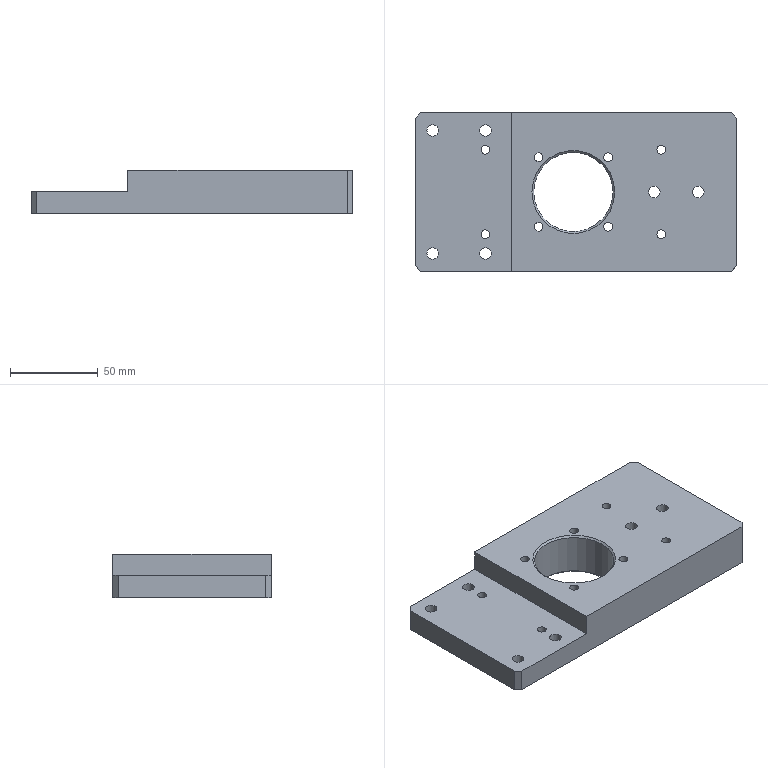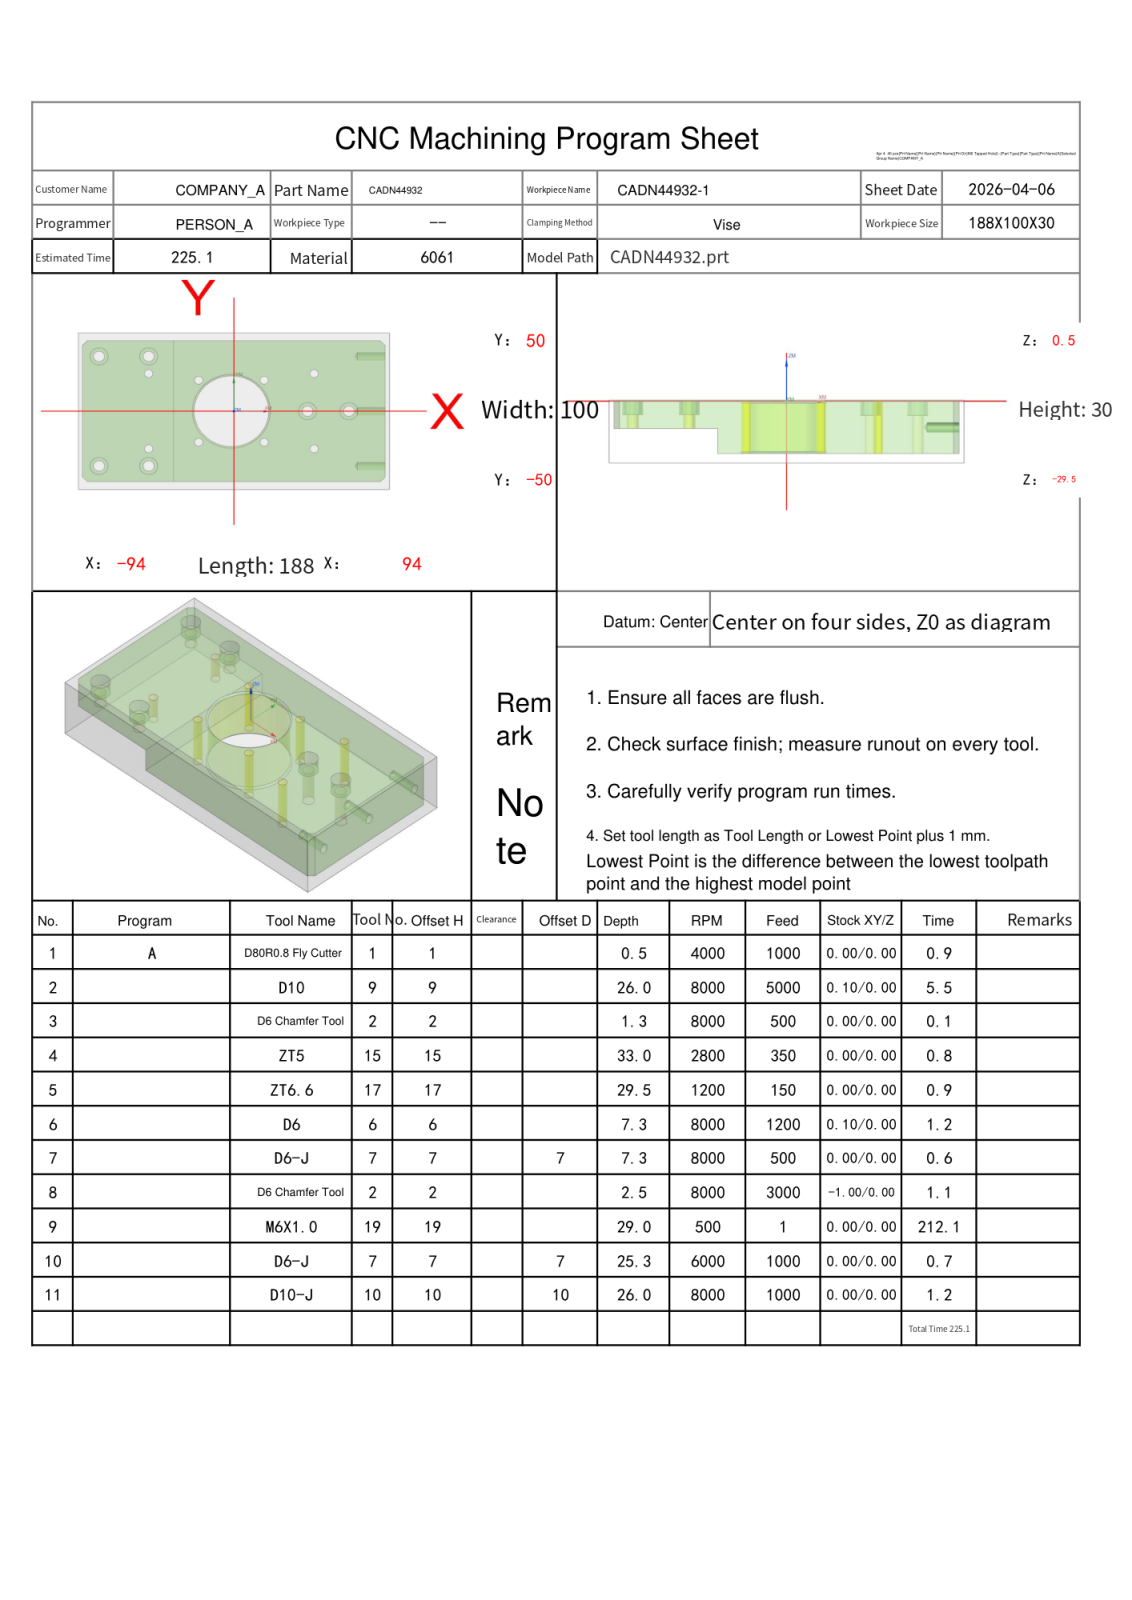NC program | NX | posted by the shop | part box 183 x 90 x 25 mm
Whole program, first 1257 of 1685 lines:
%
O0001
(Machine time: 431.06 MIN)
(===Total Tool:9===)
(T1=D80R0.8 Fly Cutter D=80.  R=0.8  D-  H01 Z=0.    )
(T9=D10     D=10.  R=0.   D-  H09 Z=-25.5 )
(T2=D6 Chamfer Tool   D=6.   R=0.   D-  H02 Z=-2.   )
(T15=ZT5    D=5.   DR_a=118 D-  H15 Z=-32.5 )
(T17=ZT6.6  D=6.6  DR_a=118 D-  H17 Z=-28.98)
(T6=D6      D=6.   R=0.   D-  H06 Z=-6.8  )
(T7=D6-J    D=6.   R=0.   D7  H07 Z=-24.8 )
(T19=M6X1.0 D=5.   DR_a=180 D-  H19 Z=-28.5 )
(T10=D10-J  D=10.  R=0.   D10 H10 Z=-25.5 )
G80 G90 G17 G49 G40
G91 G28 Z0
M01
N1 T01 M06
(D80R0.8 Fly Cutter  D=80. R=0.8 H=01 ce=0.00 di=0.00)
G00 G90 G54 X136.5 Y-42.5 M03 S4000
G43 H01 Z20.
M08
Z2.
G01 Z0.0 F1000.
X131.5
X-131.5
Y0.0
X131.5
Y42.5
X-131.5
X-136.5
Z2.
G00 Z20.
G91 G28 Z0.0
M05
M09
G91 G28 Z0.0
M01
N2 T09 M06
(D10  D=10. R=0. H=09 ce=0.10 di=0.00)
G00 G90 G54 X0.0 Y-50.1 M03 S8000
G43 H09 Z20.
M08
Z.5
G01 X-88.5 Z.378 F5000.
G02 X-92.106 Y-48.606 Z.372 I0.0 J5.1
G01 X-95.106 Y-45.606 Z.367
G02 X-96.6 Y-42. Z.361 I3.606 J3.606
G01 Y42. Z.245
G02 X-95.106 Y45.606 Z.24 I5.1 J0.0
G01 X-92.106 Y48.606 Z.234
G02 X-88.5 Y50.1 Z.228 I3.606 J-3.606
G01 X88.5 Z-.016
G02 X92.106 Y48.606 Z-.022 I0.0 J-5.1
G01 X95.106 Y45.606 Z-.027
G02 X96.6 Y42. Z-.033 I-3.606 J-3.606
G01 Y-42. Z-.149
G02 X95.106 Y-45.606 Z-.154 I-5.1 J0.0
G01 X92.106 Y-48.606 Z-.16
G02 X88.5 Y-50.1 Z-.166 I-3.606 J3.606
G01 X-88.5 Z-.41
G02 X-92.106 Y-48.606 Z-.416 I0.0 J5.1
G01 X-95.106 Y-45.606 Z-.421
G02 X-96.6 Y-42. Z-.427 I3.606 J3.606
G01 Y42. Z-.543
G02 X-95.106 Y45.606 Z-.548 I5.1 J0.0
G01 X-92.106 Y48.606 Z-.554
G02 X-88.5 Y50.1 Z-.56 I3.606 J-3.606
G01 X88.5 Z-.804
G02 X92.106 Y48.606 Z-.809 I0.0 J-5.1
G01 X95.106 Y45.606 Z-.815
G02 X96.6 Y42. Z-.821 I-3.606 J-3.606
G01 Y-42. Z-.937
G02 X95.106 Y-45.606 Z-.942 I-5.1 J0.0
G01 X92.106 Y-48.606 Z-.948
G02 X88.5 Y-50.1 Z-.954 I-3.606 J3.606
G01 X-88.5 Z-1.198
G02 X-92.106 Y-48.606 Z-1.203 I0.0 J5.1
G01 X-95.106 Y-45.606 Z-1.209
G02 X-96.6 Y-42. Z-1.215 I3.606 J3.606
G01 Y42. Z-1.331
G02 X-95.106 Y45.606 Z-1.336 I5.1 J0.0
G01 X-92.106 Y48.606 Z-1.342
G02 X-88.5 Y50.1 Z-1.348 I3.606 J-3.606
G01 X88.5 Z-1.592
G02 X92.106 Y48.606 Z-1.597 I0.0 J-5.1
G01 X95.106 Y45.606 Z-1.603
G02 X96.6 Y42. Z-1.609 I-3.606 J-3.606
G01 Y-42. Z-1.725
G02 X95.106 Y-45.606 Z-1.73 I-5.1 J0.0
G01 X92.106 Y-48.606 Z-1.736
G02 X88.5 Y-50.1 Z-1.742 I-3.606 J3.606
G01 X-88.5 Z-1.986
G02 X-92.106 Y-48.606 Z-1.991 I0.0 J5.1
G01 X-95.106 Y-45.606 Z-1.997
G02 X-96.6 Y-42. Z-2.003 I3.606 J3.606
G01 Y42. Z-2.119
G02 X-95.106 Y45.606 Z-2.124 I5.1 J0.0
G01 X-92.106 Y48.606 Z-2.13
G02 X-88.5 Y50.1 Z-2.135 I3.606 J-3.606
G01 X88.5 Z-2.38
G02 X92.106 Y48.606 Z-2.385 I0.0 J-5.1
G01 X95.106 Y45.606 Z-2.391
G02 X96.6 Y42. Z-2.397 I-3.606 J-3.606
G01 Y-42. Z-2.512
G02 X95.106 Y-45.606 Z-2.518 I-5.1 J0.0
G01 X92.106 Y-48.606 Z-2.524
G02 X88.5 Y-50.1 Z-2.529 I-3.606 J3.606
G01 X-88.5 Z-2.774
G02 X-92.106 Y-48.606 Z-2.779 I0.0 J5.1
G01 X-95.106 Y-45.606 Z-2.785
G02 X-96.6 Y-42. Z-2.791 I3.606 J3.606
G01 Y42. Z-2.906
G02 X-95.106 Y45.606 Z-2.912 I5.1 J0.0
G01 X-92.106 Y48.606 Z-2.918
G02 X-88.5 Y50.1 Z-2.923 I3.606 J-3.606
G01 X88.5 Z-3.168
G02 X92.106 Y48.606 Z-3.173 I0.0 J-5.1
G01 X95.106 Y45.606 Z-3.179
G02 X96.6 Y42. Z-3.184 I-3.606 J-3.606
G01 Y-42. Z-3.3
G02 X95.106 Y-45.606 Z-3.306 I-5.1 J0.0
G01 X92.106 Y-48.606 Z-3.312
G02 X88.5 Y-50.1 Z-3.317 I-3.606 J3.606
G01 X-88.5 Z-3.562
G02 X-92.106 Y-48.606 Z-3.567 I0.0 J5.1
G01 X-95.106 Y-45.606 Z-3.573
G02 X-96.6 Y-42. Z-3.578 I3.606 J3.606
G01 Y42. Z-3.694
G02 X-95.106 Y45.606 Z-3.7 I5.1 J0.0
G01 X-92.106 Y48.606 Z-3.706
G02 X-88.5 Y50.1 Z-3.711 I3.606 J-3.606
G01 X88.5 Z-3.955
G02 X92.106 Y48.606 Z-3.961 I0.0 J-5.1
G01 X95.106 Y45.606 Z-3.967
G02 X96.6 Y42. Z-3.972 I-3.606 J-3.606
G01 Y-42. Z-4.088
G02 X95.106 Y-45.606 Z-4.094 I-5.1 J0.0
G01 X92.106 Y-48.606 Z-4.1
G02 X88.5 Y-50.1 Z-4.105 I-3.606 J3.606
G01 X-88.5 Z-4.349
G02 X-92.106 Y-48.606 Z-4.355 I0.0 J5.1
G01 X-95.106 Y-45.606 Z-4.361
G02 X-96.6 Y-42. Z-4.366 I3.606 J3.606
G01 Y42. Z-4.482
G02 X-95.106 Y45.606 Z-4.488 I5.1 J0.0
G01 X-92.106 Y48.606 Z-4.494
G02 X-88.5 Y50.1 Z-4.499 I3.606 J-3.606
G01 X88.5 Z-4.743
G02 X92.106 Y48.606 Z-4.749 I0.0 J-5.1
G01 X95.106 Y45.606 Z-4.755
G02 X96.6 Y42. Z-4.76 I-3.606 J-3.606
G01 Y-42. Z-4.876
G02 X95.106 Y-45.606 Z-4.882 I-5.1 J0.0
G01 X92.106 Y-48.606 Z-4.888
G02 X88.5 Y-50.1 Z-4.893 I-3.606 J3.606
G01 X-88.5 Z-5.137
G02 X-92.106 Y-48.606 Z-5.143 I0.0 J5.1
G01 X-95.106 Y-45.606 Z-5.149
G02 X-96.6 Y-42. Z-5.154 I3.606 J3.606
G01 Y42. Z-5.27
G02 X-95.106 Y45.606 Z-5.276 I5.1 J0.0
G01 X-92.106 Y48.606 Z-5.281
G02 X-88.5 Y50.1 Z-5.287 I3.606 J-3.606
G01 X88.5 Z-5.531
G02 X92.106 Y48.606 Z-5.537 I0.0 J-5.1
G01 X95.106 Y45.606 Z-5.543
G02 X96.6 Y42. Z-5.548 I-3.606 J-3.606
G01 Y-42. Z-5.664
G02 X95.106 Y-45.606 Z-5.67 I-5.1 J0.0
G01 X92.106 Y-48.606 Z-5.675
G02 X88.5 Y-50.1 Z-5.681 I-3.606 J3.606
G01 X-88.5 Z-5.925
G02 X-92.106 Y-48.606 Z-5.931 I0.0 J5.1
G01 X-95.106 Y-45.606 Z-5.937
G02 X-96.6 Y-42. Z-5.942 I3.606 J3.606
G01 Y42. Z-6.058
G02 X-95.106 Y45.606 Z-6.063 I5.1 J0.0
G01 X-92.106 Y48.606 Z-6.069
G02 X-88.5 Y50.1 Z-6.075 I3.606 J-3.606
G01 X88.5 Z-6.319
G02 X92.106 Y48.606 Z-6.325 I0.0 J-5.1
G01 X95.106 Y45.606 Z-6.33
G02 X96.6 Y42. Z-6.336 I-3.606 J-3.606
G01 Y-42. Z-6.452
G02 X95.106 Y-45.606 Z-6.457 I-5.1 J0.0
G01 X92.106 Y-48.606 Z-6.463
G02 X88.5 Y-50.1 Z-6.469 I-3.606 J3.606
G01 X-88.5 Z-6.713
G02 X-92.106 Y-48.606 Z-6.719 I0.0 J5.1
G01 X-95.106 Y-45.606 Z-6.724
G02 X-96.6 Y-42. Z-6.73 I3.606 J3.606
G01 Y42. Z-6.846
G02 X-95.106 Y45.606 Z-6.851 I5.1 J0.0
G01 X-92.106 Y48.606 Z-6.857
G02 X-88.5 Y50.1 Z-6.863 I3.606 J-3.606
G01 X88.5 Z-7.107
G02 X92.106 Y48.606 Z-7.112 I0.0 J-5.1
G01 X95.106 Y45.606 Z-7.118
G02 X96.6 Y42. Z-7.124 I-3.606 J-3.606
G01 Y-42. Z-7.24
G02 X95.106 Y-45.606 Z-7.245 I-5.1 J0.0
G01 X92.106 Y-48.606 Z-7.251
G02 X88.5 Y-50.1 Z-7.257 I-3.606 J3.606
G01 X-88.5 Z-7.501
G02 X-92.106 Y-48.606 Z-7.506 I0.0 J5.1
G01 X-95.106 Y-45.606 Z-7.512
G02 X-96.6 Y-42. Z-7.518 I3.606 J3.606
G01 Y42. Z-7.634
G02 X-95.106 Y45.606 Z-7.639 I5.1 J0.0
G01 X-92.106 Y48.606 Z-7.645
G02 X-88.5 Y50.1 Z-7.651 I3.606 J-3.606
G01 X88.5 Z-7.895
G02 X92.106 Y48.606 Z-7.9 I0.0 J-5.1
G01 X95.106 Y45.606 Z-7.906
G02 X96.6 Y42. Z-7.912 I-3.606 J-3.606
G01 Y-42. Z-8.028
G02 X95.106 Y-45.606 Z-8.033 I-5.1 J0.0
G01 X92.106 Y-48.606 Z-8.039
G02 X88.5 Y-50.1 Z-8.045 I-3.606 J3.606
G01 X-88.5 Z-8.289
G02 X-92.106 Y-48.606 Z-8.294 I0.0 J5.1
G01 X-95.106 Y-45.606 Z-8.3
G02 X-96.6 Y-42. Z-8.306 I3.606 J3.606
G01 Y42. Z-8.422
G02 X-95.106 Y45.606 Z-8.427 I5.1 J0.0
G01 X-92.106 Y48.606 Z-8.433
G02 X-88.5 Y50.1 Z-8.438 I3.606 J-3.606
G01 X88.5 Z-8.683
G02 X92.106 Y48.606 Z-8.688 I0.0 J-5.1
G01 X95.106 Y45.606 Z-8.694
G02 X96.6 Y42. Z-8.7 I-3.606 J-3.606
G01 Y-42. Z-8.816
G02 X95.106 Y-45.606 Z-8.821 I-5.1 J0.0
G01 X92.106 Y-48.606 Z-8.827
G02 X88.5 Y-50.1 Z-8.832 I-3.606 J3.606
G01 X-88.5 Z-9.077
G02 X-92.106 Y-48.606 Z-9.082 I0.0 J5.1
G01 X-95.106 Y-45.606 Z-9.088
G02 X-96.6 Y-42. Z-9.094 I3.606 J3.606
G01 Y42. Z-9.209
G02 X-95.106 Y45.606 Z-9.215 I5.1 J0.0
G01 X-92.106 Y48.606 Z-9.221
G02 X-88.5 Y50.1 Z-9.226 I3.606 J-3.606
G01 X88.5 Z-9.471
G02 X92.106 Y48.606 Z-9.476 I0.0 J-5.1
G01 X95.106 Y45.606 Z-9.482
G02 X96.6 Y42. Z-9.488 I-3.606 J-3.606
G01 Y-42. Z-9.603
G02 X95.106 Y-45.606 Z-9.609 I-5.1 J0.0
G01 X92.106 Y-48.606 Z-9.615
G02 X88.5 Y-50.1 Z-9.62 I-3.606 J3.606
G01 X-88.5 Z-9.865
G02 X-92.106 Y-48.606 Z-9.87 I0.0 J5.1
G01 X-95.106 Y-45.606 Z-9.876
G02 X-96.6 Y-42. Z-9.881 I3.606 J3.606
G01 Y42. Z-9.997
G02 X-95.106 Y45.606 Z-10.003 I5.1 J0.0
G01 X-92.106 Y48.606 Z-10.009
G02 X-88.5 Y50.1 Z-10.014 I3.606 J-3.606
G01 X88.5 Z-10.258
G02 X92.106 Y48.606 Z-10.264 I0.0 J-5.1
G01 X95.106 Y45.606 Z-10.27
G02 X96.6 Y42. Z-10.275 I-3.606 J-3.606
G01 Y-42. Z-10.391
G02 X95.106 Y-45.606 Z-10.397 I-5.1 J0.0
G01 X92.106 Y-48.606 Z-10.403
G02 X88.5 Y-50.1 Z-10.408 I-3.606 J3.606
G01 X-88.5 Z-10.652
G02 X-92.106 Y-48.606 Z-10.658 I0.0 J5.1
G01 X-95.106 Y-45.606 Z-10.664
G02 X-96.6 Y-42. Z-10.669 I3.606 J3.606
G01 Y42. Z-10.785
G02 X-95.106 Y45.606 Z-10.791 I5.1 J0.0
G01 X-92.106 Y48.606 Z-10.797
G02 X-88.5 Y50.1 Z-10.802 I3.606 J-3.606
G01 X88.5 Z-11.046
G02 X92.106 Y48.606 Z-11.052 I0.0 J-5.1
G01 X95.106 Y45.606 Z-11.058
G02 X96.6 Y42. Z-11.063 I-3.606 J-3.606
G01 Y-42. Z-11.179
G02 X95.106 Y-45.606 Z-11.185 I-5.1 J0.0
G01 X92.106 Y-48.606 Z-11.191
G02 X88.5 Y-50.1 Z-11.196 I-3.606 J3.606
G01 X-88.5 Z-11.44
G02 X-92.106 Y-48.606 Z-11.446 I0.0 J5.1
G01 X-95.106 Y-45.606 Z-11.452
G02 X-96.6 Y-42. Z-11.457 I3.606 J3.606
G01 Y42. Z-11.573
G02 X-95.106 Y45.606 Z-11.579 I5.1 J0.0
G01 X-92.106 Y48.606 Z-11.584
G02 X-88.5 Y50.1 Z-11.59 I3.606 J-3.606
G01 X88.5 Z-11.834
G02 X92.106 Y48.606 Z-11.84 I0.0 J-5.1
G01 X95.106 Y45.606 Z-11.846
G02 X96.6 Y42. Z-11.851 I-3.606 J-3.606
G01 Y-42. Z-11.967
G02 X95.106 Y-45.606 Z-11.973 I-5.1 J0.0
G01 X92.106 Y-48.606 Z-11.978
G02 X88.5 Y-50.1 Z-11.984 I-3.606 J3.606
G01 X-88.5 Z-12.228
G02 X-92.106 Y-48.606 Z-12.234 I0.0 J5.1
G01 X-95.106 Y-45.606 Z-12.24
G02 X-96.6 Y-42. Z-12.245 I3.606 J3.606
G01 Y42. Z-12.361
G02 X-95.106 Y45.606 Z-12.367 I5.1 J0.0
G01 X-92.106 Y48.606 Z-12.372
G02 X-88.5 Y50.1 Z-12.378 I3.606 J-3.606
G01 X88.5 Z-12.622
G02 X92.106 Y48.606 Z-12.628 I0.0 J-5.1
G01 X95.106 Y45.606 Z-12.633
G02 X96.6 Y42. Z-12.639 I-3.606 J-3.606
G01 Y-42. Z-12.755
G02 X95.106 Y-45.606 Z-12.76 I-5.1 J0.0
G01 X92.106 Y-48.606 Z-12.766
G02 X88.5 Y-50.1 Z-12.772 I-3.606 J3.606
G01 X-88.5 Z-13.016
G02 X-92.106 Y-48.606 Z-13.022 I0.0 J5.1
G01 X-95.106 Y-45.606 Z-13.027
G02 X-96.6 Y-42. Z-13.033 I3.606 J3.606
G01 Y42. Z-13.149
G02 X-95.106 Y45.606 Z-13.154 I5.1 J0.0
G01 X-92.106 Y48.606 Z-13.16
G02 X-88.5 Y50.1 Z-13.166 I3.606 J-3.606
G01 X88.5 Z-13.41
G02 X92.106 Y48.606 Z-13.416 I0.0 J-5.1
G01 X95.106 Y45.606 Z-13.421
G02 X96.6 Y42. Z-13.427 I-3.606 J-3.606
G01 Y-42. Z-13.543
G02 X95.106 Y-45.606 Z-13.548 I-5.1 J0.0
G01 X92.106 Y-48.606 Z-13.554
G02 X88.5 Y-50.1 Z-13.56 I-3.606 J3.606
G01 X-88.5 Z-13.804
G02 X-92.106 Y-48.606 Z-13.809 I0.0 J5.1
G01 X-95.106 Y-45.606 Z-13.815
G02 X-96.6 Y-42. Z-13.821 I3.606 J3.606
G01 Y42. Z-13.937
G02 X-95.106 Y45.606 Z-13.942 I5.1 J0.0
G01 X-92.106 Y48.606 Z-13.948
G02 X-88.5 Y50.1 Z-13.954 I3.606 J-3.606
G01 X88.5 Z-14.198
G02 X92.106 Y48.606 Z-14.203 I0.0 J-5.1
G01 X95.106 Y45.606 Z-14.209
G02 X96.6 Y42. Z-14.215 I-3.606 J-3.606
G01 Y-42. Z-14.331
G02 X95.106 Y-45.606 Z-14.336 I-5.1 J0.0
G01 X92.106 Y-48.606 Z-14.342
G02 X88.5 Y-50.1 Z-14.348 I-3.606 J3.606
G01 X-88.5 Z-14.592
G02 X-92.106 Y-48.606 Z-14.597 I0.0 J5.1
G01 X-95.106 Y-45.606 Z-14.603
G02 X-96.6 Y-42. Z-14.609 I3.606 J3.606
G01 Y42. Z-14.725
G02 X-95.106 Y45.606 Z-14.73 I5.1 J0.0
G01 X-92.106 Y48.606 Z-14.736
G02 X-88.5 Y50.1 Z-14.742 I3.606 J-3.606
G01 X88.5 Z-14.986
G02 X92.106 Y48.606 Z-14.991 I0.0 J-5.1
G01 X95.106 Y45.606 Z-14.997
G02 X96.6 Y42. Z-15.003 I-3.606 J-3.606
G01 Y-42. Z-15.119
G02 X95.106 Y-45.606 Z-15.124 I-5.1 J0.0
G01 X92.106 Y-48.606 Z-15.13
G02 X88.5 Y-50.1 Z-15.135 I-3.606 J3.606
G01 X-88.5 Z-15.38
G02 X-92.106 Y-48.606 Z-15.385 I0.0 J5.1
G01 X-95.106 Y-45.606 Z-15.391
G02 X-96.6 Y-42. Z-15.397 I3.606 J3.606
G01 Y42. Z-15.512
G02 X-95.106 Y45.606 Z-15.518 I5.1 J0.0
G01 X-92.106 Y48.606 Z-15.524
G02 X-88.5 Y50.1 Z-15.529 I3.606 J-3.606
G01 X88.5 Z-15.774
G02 X92.106 Y48.606 Z-15.779 I0.0 J-5.1
G01 X95.106 Y45.606 Z-15.785
G02 X96.6 Y42. Z-15.791 I-3.606 J-3.606
G01 Y-42. Z-15.906
G02 X95.106 Y-45.606 Z-15.912 I-5.1 J0.0
G01 X92.106 Y-48.606 Z-15.918
G02 X88.5 Y-50.1 Z-15.923 I-3.606 J3.606
G01 X-88.5 Z-16.168
G02 X-92.106 Y-48.606 Z-16.173 I0.0 J5.1
G01 X-95.106 Y-45.606 Z-16.179
G02 X-96.6 Y-42. Z-16.184 I3.606 J3.606
G01 Y42. Z-16.3
G02 X-95.106 Y45.606 Z-16.306 I5.1 J0.0
G01 X-92.106 Y48.606 Z-16.312
G02 X-88.5 Y50.1 Z-16.317 I3.606 J-3.606
G01 X88.5 Z-16.562
G02 X92.106 Y48.606 Z-16.567 I0.0 J-5.1
G01 X95.106 Y45.606 Z-16.573
G02 X96.6 Y42. Z-16.578 I-3.606 J-3.606
G01 Y-42. Z-16.694
G02 X95.106 Y-45.606 Z-16.7 I-5.1 J0.0
G01 X92.106 Y-48.606 Z-16.706
G02 X88.5 Y-50.1 Z-16.711 I-3.606 J3.606
G01 X-88.5 Z-16.955
G02 X-92.106 Y-48.606 Z-16.961 I0.0 J5.1
G01 X-95.106 Y-45.606 Z-16.967
G02 X-96.6 Y-42. Z-16.972 I3.606 J3.606
G01 Y42. Z-17.088
G02 X-95.106 Y45.606 Z-17.094 I5.1 J0.0
G01 X-92.106 Y48.606 Z-17.1
G02 X-88.5 Y50.1 Z-17.105 I3.606 J-3.606
G01 X88.5 Z-17.349
G02 X92.106 Y48.606 Z-17.355 I0.0 J-5.1
G01 X95.106 Y45.606 Z-17.361
G02 X96.6 Y42. Z-17.366 I-3.606 J-3.606
G01 Y-42. Z-17.482
G02 X95.106 Y-45.606 Z-17.488 I-5.1 J0.0
G01 X92.106 Y-48.606 Z-17.494
G02 X88.5 Y-50.1 Z-17.499 I-3.606 J3.606
G01 X-88.5 Z-17.743
G02 X-92.106 Y-48.606 Z-17.749 I0.0 J5.1
G01 X-95.106 Y-45.606 Z-17.755
G02 X-96.6 Y-42. Z-17.76 I3.606 J3.606
G01 Y42. Z-17.876
G02 X-95.106 Y45.606 Z-17.882 I5.1 J0.0
G01 X-92.106 Y48.606 Z-17.888
G02 X-88.5 Y50.1 Z-17.893 I3.606 J-3.606
G01 X88.5 Z-18.137
G02 X92.106 Y48.606 Z-18.143 I0.0 J-5.1
G01 X95.106 Y45.606 Z-18.149
G02 X96.6 Y42. Z-18.154 I-3.606 J-3.606
G01 Y-42. Z-18.27
G02 X95.106 Y-45.606 Z-18.276 I-5.1 J0.0
G01 X92.106 Y-48.606 Z-18.281
G02 X88.5 Y-50.1 Z-18.287 I-3.606 J3.606
G01 X-88.5 Z-18.531
G02 X-92.106 Y-48.606 Z-18.537 I0.0 J5.1
G01 X-95.106 Y-45.606 Z-18.543
G02 X-96.6 Y-42. Z-18.548 I3.606 J3.606
G01 Y42. Z-18.664
G02 X-95.106 Y45.606 Z-18.67 I5.1 J0.0
G01 X-92.106 Y48.606 Z-18.675
G02 X-88.5 Y50.1 Z-18.681 I3.606 J-3.606
G01 X88.5 Z-18.925
G02 X92.106 Y48.606 Z-18.931 I0.0 J-5.1
G01 X95.106 Y45.606 Z-18.937
G02 X96.6 Y42. Z-18.942 I-3.606 J-3.606
G01 Y-42. Z-19.058
G02 X95.106 Y-45.606 Z-19.063 I-5.1 J0.0
G01 X92.106 Y-48.606 Z-19.069
G02 X88.5 Y-50.1 Z-19.075 I-3.606 J3.606
G01 X-88.5 Z-19.319
G02 X-92.106 Y-48.606 Z-19.325 I0.0 J5.1
G01 X-95.106 Y-45.606 Z-19.33
G02 X-96.6 Y-42. Z-19.336 I3.606 J3.606
G01 Y42. Z-19.452
G02 X-95.106 Y45.606 Z-19.457 I5.1 J0.0
G01 X-92.106 Y48.606 Z-19.463
G02 X-88.5 Y50.1 Z-19.469 I3.606 J-3.606
G01 X88.5 Z-19.713
G02 X92.106 Y48.606 Z-19.719 I0.0 J-5.1
G01 X95.106 Y45.606 Z-19.724
G02 X96.6 Y42. Z-19.73 I-3.606 J-3.606
G01 Y-42. Z-19.846
G02 X95.106 Y-45.606 Z-19.851 I-5.1 J0.0
G01 X92.106 Y-48.606 Z-19.857
G02 X88.5 Y-50.1 Z-19.863 I-3.606 J3.606
G01 X-88.5 Z-20.107
G02 X-92.106 Y-48.606 Z-20.112 I0.0 J5.1
G01 X-95.106 Y-45.606 Z-20.118
G02 X-96.6 Y-42. Z-20.124 I3.606 J3.606
G01 Y42. Z-20.24
G02 X-95.106 Y45.606 Z-20.245 I5.1 J0.0
G01 X-92.106 Y48.606 Z-20.251
G02 X-88.5 Y50.1 Z-20.257 I3.606 J-3.606
G01 X88.5 Z-20.501
G02 X92.106 Y48.606 Z-20.506 I0.0 J-5.1
G01 X95.106 Y45.606 Z-20.512
G02 X96.6 Y42. Z-20.518 I-3.606 J-3.606
G01 Y-42. Z-20.634
G02 X95.106 Y-45.606 Z-20.639 I-5.1 J0.0
G01 X92.106 Y-48.606 Z-20.645
G02 X88.5 Y-50.1 Z-20.651 I-3.606 J3.606
G01 X-88.5 Z-20.895
G02 X-92.106 Y-48.606 Z-20.9 I0.0 J5.1
G01 X-95.106 Y-45.606 Z-20.906
G02 X-96.6 Y-42. Z-20.912 I3.606 J3.606
G01 Y42. Z-21.028
G02 X-95.106 Y45.606 Z-21.033 I5.1 J0.0
G01 X-92.106 Y48.606 Z-21.039
G02 X-88.5 Y50.1 Z-21.045 I3.606 J-3.606
G01 X88.5 Z-21.289
G02 X92.106 Y48.606 Z-21.294 I0.0 J-5.1
G01 X95.106 Y45.606 Z-21.3
G02 X96.6 Y42. Z-21.306 I-3.606 J-3.606
G01 Y-42. Z-21.422
G02 X95.106 Y-45.606 Z-21.427 I-5.1 J0.0
G01 X92.106 Y-48.606 Z-21.433
G02 X88.5 Y-50.1 Z-21.438 I-3.606 J3.606
G01 X-88.5 Z-21.683
G02 X-92.106 Y-48.606 Z-21.688 I0.0 J5.1
G01 X-95.106 Y-45.606 Z-21.694
G02 X-96.6 Y-42. Z-21.7 I3.606 J3.606
G01 Y42. Z-21.816
G02 X-95.106 Y45.606 Z-21.821 I5.1 J0.0
G01 X-92.106 Y48.606 Z-21.827
G02 X-88.5 Y50.1 Z-21.832 I3.606 J-3.606
G01 X88.5 Z-22.077
G02 X92.106 Y48.606 Z-22.082 I0.0 J-5.1
G01 X95.106 Y45.606 Z-22.088
G02 X96.6 Y42. Z-22.094 I-3.606 J-3.606
G01 Y-42. Z-22.209
G02 X95.106 Y-45.606 Z-22.215 I-5.1 J0.0
G01 X92.106 Y-48.606 Z-22.221
G02 X88.5 Y-50.1 Z-22.226 I-3.606 J3.606
G01 X-88.5 Z-22.471
G02 X-92.106 Y-48.606 Z-22.476 I0.0 J5.1
G01 X-95.106 Y-45.606 Z-22.482
G02 X-96.6 Y-42. Z-22.488 I3.606 J3.606
G01 Y42. Z-22.603
G02 X-95.106 Y45.606 Z-22.609 I5.1 J0.0
G01 X-92.106 Y48.606 Z-22.615
G02 X-88.5 Y50.1 Z-22.62 I3.606 J-3.606
G01 X88.5 Z-22.865
G02 X92.106 Y48.606 Z-22.87 I0.0 J-5.1
G01 X95.106 Y45.606 Z-22.876
G02 X96.6 Y42. Z-22.881 I-3.606 J-3.606
G01 Y-42. Z-22.997
G02 X95.106 Y-45.606 Z-23.003 I-5.1 J0.0
G01 X92.106 Y-48.606 Z-23.009
G02 X88.5 Y-50.1 Z-23.014 I-3.606 J3.606
G01 X-88.5 Z-23.258
G02 X-92.106 Y-48.606 Z-23.264 I0.0 J5.1
G01 X-95.106 Y-45.606 Z-23.27
G02 X-96.6 Y-42. Z-23.275 I3.606 J3.606
G01 Y42. Z-23.391
G02 X-95.106 Y45.606 Z-23.397 I5.1 J0.0
G01 X-92.106 Y48.606 Z-23.403
G02 X-88.5 Y50.1 Z-23.408 I3.606 J-3.606
G01 X88.5 Z-23.652
G02 X92.106 Y48.606 Z-23.658 I0.0 J-5.1
G01 X95.106 Y45.606 Z-23.664
G02 X96.6 Y42. Z-23.669 I-3.606 J-3.606
G01 Y-42. Z-23.785
G02 X95.106 Y-45.606 Z-23.791 I-5.1 J0.0
G01 X92.106 Y-48.606 Z-23.797
G02 X88.5 Y-50.1 Z-23.802 I-3.606 J3.606
G01 X-88.5 Z-24.046
G02 X-92.106 Y-48.606 Z-24.052 I0.0 J5.1
G01 X-95.106 Y-45.606 Z-24.058
G02 X-96.6 Y-42. Z-24.063 I3.606 J3.606
G01 Y42. Z-24.179
G02 X-95.106 Y45.606 Z-24.185 I5.1 J0.0
G01 X-92.106 Y48.606 Z-24.191
G02 X-88.5 Y50.1 Z-24.196 I3.606 J-3.606
G01 X88.5 Z-24.44
G02 X92.106 Y48.606 Z-24.446 I0.0 J-5.1
G01 X95.106 Y45.606 Z-24.452
G02 X96.6 Y42. Z-24.457 I-3.606 J-3.606
G01 Y-42. Z-24.573
G02 X95.106 Y-45.606 Z-24.579 I-5.1 J0.0
G01 X92.106 Y-48.606 Z-24.584
G02 X88.5 Y-50.1 Z-24.59 I-3.606 J3.606
G01 X-88.5 Z-24.834
G02 X-92.106 Y-48.606 Z-24.84 I0.0 J5.1
G01 X-95.106 Y-45.606 Z-24.846
G02 X-96.6 Y-42. Z-24.851 I3.606 J3.606
G01 Y42. Z-24.967
G02 X-95.106 Y45.606 Z-24.973 I5.1 J0.0
G01 X-92.106 Y48.606 Z-24.978
G02 X-88.5 Y50.1 Z-24.984 I3.606 J-3.606
G01 X88.5 Z-25.228
G02 X92.106 Y48.606 Z-25.234 I0.0 J-5.1
G01 X95.106 Y45.606 Z-25.24
G02 X96.6 Y42. Z-25.245 I-3.606 J-3.606
G01 Y-42. Z-25.361
G02 X95.106 Y-45.606 Z-25.367 I-5.1 J0.0
G01 X92.106 Y-48.606 Z-25.372
G02 X88.5 Y-50.1 Z-25.378 I-3.606 J3.606
G01 X0.0 Z-25.5
X-88.5
G02 X-92.106 Y-48.606 I0.0 J5.1
G01 X-95.106 Y-45.606
G02 X-96.6 Y-42. I3.606 J3.606
G01 Y42.
G02 X-95.106 Y45.606 I5.1 J0.0
G01 X-92.106 Y48.606
G02 X-88.5 Y50.1 I3.606 J-3.606
G01 X88.5
G02 X92.106 Y48.606 I0.0 J-5.1
G01 X95.106 Y45.606
G02 X96.6 Y42. I-3.606 J-3.606
G01 Y-42.
G02 X95.106 Y-45.606 I-5.1 J0.0
G01 X92.106 Y-48.606
G02 X88.5 Y-50.1 I-3.606 J3.606
G01 X0.0
X-.5
Z-24.5
G00 Z20.
G00 G90 X13.972 Y8.017 M03 S8000
Z20.
Z1.
G01 X13.465 Y9.034 Z.94 F3000.
X11.817 Y11.323 Z.793
X9.823 Y13.317 Z.645
X7.534 Y14.965 Z.497
X5.01 Y16.223 Z.349
X2.316 Y17.058 Z.201
X-.476 Y17.45 Z.054
X-1.5 Z0.0
G03 X-18.95 Y0.0 Z-.148 I0.0 J-17.45
X-1.5 Y-17.45 Z-.295 I17.45 J0.0
X15.95 Y0.0 Z-.443 I0.0 J17.45
X-1.5 Y17.45 Z-.59 I-17.45 J0.0
X-18.95 Y0.0 Z-.738 I0.0 J-17.45
X-1.5 Y-17.45 Z-.886 I17.45 J0.0
X15.95 Y0.0 Z-1.033 I0.0 J17.45
X-1.5 Y17.45 Z-1.181 I-17.45 J0.0
X-18.95 Y0.0 Z-1.329 I0.0 J-17.45
X-1.5 Y-17.45 Z-1.476 I17.45 J0.0
X15.95 Y0.0 Z-1.624 I0.0 J17.45
X-1.5 Y17.45 Z-1.771 I-17.45 J0.0
X-18.95 Y0.0 Z-1.919 I0.0 J-17.45
X-1.5 Y-17.45 Z-2.067 I17.45 J0.0
X15.95 Y0.0 Z-2.214 I0.0 J17.45
X-1.5 Y17.45 Z-2.362 I-17.45 J0.0
X-18.95 Y0.0 Z-2.51 I0.0 J-17.45
X-1.5 Y-17.45 Z-2.657 I17.45 J0.0
X15.95 Y0.0 Z-2.805 I0.0 J17.45
X-1.5 Y17.45 Z-2.952 I-17.45 J0.0
X-18.95 Y0.0 Z-3.1 I0.0 J-17.45
X-1.5 Y-17.45 Z-3.248 I17.45 J0.0
X15.95 Y0.0 Z-3.395 I0.0 J17.45
X-1.5 Y17.45 Z-3.543 I-17.45 J0.0
X-18.95 Y0.0 Z-3.69 I0.0 J-17.45
X-1.5 Y-17.45 Z-3.838 I17.45 J0.0
X15.95 Y0.0 Z-3.986 I0.0 J17.45
X-1.5 Y17.45 Z-4.133 I-17.45 J0.0
X-18.95 Y0.0 Z-4.281 I0.0 J-17.45
X-1.5 Y-17.45 Z-4.429 I17.45 J0.0
X15.95 Y0.0 Z-4.576 I0.0 J17.45
X-1.5 Y17.45 Z-4.724 I-17.45 J0.0
X-18.95 Y0.0 Z-4.871 I0.0 J-17.45
X-1.5 Y-17.45 Z-5.019 I17.45 J0.0
X15.95 Y0.0 Z-5.167 I0.0 J17.45
X-1.5 Y17.45 Z-5.314 I-17.45 J0.0
X-18.95 Y0.0 Z-5.462 I0.0 J-17.45
X-1.5 Y-17.45 Z-5.61 I17.45 J0.0
X15.95 Y0.0 Z-5.757 I0.0 J17.45
X-1.5 Y17.45 Z-5.905 I-17.45 J0.0
X-18.95 Y0.0 Z-6.052 I0.0 J-17.45
X-1.5 Y-17.45 Z-6.2 I17.45 J0.0
X15.95 Y0.0 Z-6.348 I0.0 J17.45
X-1.5 Y17.45 Z-6.495 I-17.45 J0.0
X-18.95 Y0.0 Z-6.643 I0.0 J-17.45
X-1.5 Y-17.45 Z-6.79 I17.45 J0.0
X15.95 Y0.0 Z-6.938 I0.0 J17.45
X-1.5 Y17.45 Z-7.086 I-17.45 J0.0
X-18.95 Y0.0 Z-7.233 I0.0 J-17.45
X-1.5 Y-17.45 Z-7.381 I17.45 J0.0
X15.95 Y0.0 Z-7.529 I0.0 J17.45
X-1.5 Y17.45 Z-7.676 I-17.45 J0.0
X-18.95 Y0.0 Z-7.824 I0.0 J-17.45
X-1.5 Y-17.45 Z-7.971 I17.45 J0.0
X15.95 Y0.0 Z-8.119 I0.0 J17.45
X-1.5 Y17.45 Z-8.267 I-17.45 J0.0
X-18.95 Y0.0 Z-8.414 I0.0 J-17.45
X-1.5 Y-17.45 Z-8.562 I17.45 J0.0
X15.95 Y0.0 Z-8.71 I0.0 J17.45
X-1.5 Y17.45 Z-8.857 I-17.45 J0.0
X-18.95 Y0.0 Z-9.005 I0.0 J-17.45
X-1.5 Y-17.45 Z-9.152 I17.45 J0.0
X15.95 Y0.0 Z-9.3 I0.0 J17.45
X-1.5 Y17.45 Z-9.448 I-17.45 J0.0
X-18.95 Y0.0 Z-9.595 I0.0 J-17.45
X-1.5 Y-17.45 Z-9.743 I17.45 J0.0
X15.95 Y0.0 Z-9.89 I0.0 J17.45
X-1.5 Y17.45 Z-10.038 I-17.45 J0.0
X-18.95 Y0.0 Z-10.186 I0.0 J-17.45
X-1.5 Y-17.45 Z-10.333 I17.45 J0.0
X15.95 Y0.0 Z-10.481 I0.0 J17.45
X-1.5 Y17.45 Z-10.629 I-17.45 J0.0
X-18.95 Y0.0 Z-10.776 I0.0 J-17.45
X-1.5 Y-17.45 Z-10.924 I17.45 J0.0
X15.95 Y0.0 Z-11.071 I0.0 J17.45
X-1.5 Y17.45 Z-11.219 I-17.45 J0.0
X-18.95 Y0.0 Z-11.367 I0.0 J-17.45
X-1.5 Y-17.45 Z-11.514 I17.45 J0.0
X15.95 Y0.0 Z-11.662 I0.0 J17.45
X-1.5 Y17.45 Z-11.81 I-17.45 J0.0
X-18.95 Y0.0 Z-11.957 I0.0 J-17.45
X-1.5 Y-17.45 Z-12.105 I17.45 J0.0
X15.95 Y0.0 Z-12.252 I0.0 J17.45
X-1.5 Y17.45 Z-12.4 I-17.45 J0.0
X-18.95 Y0.0 Z-12.548 I0.0 J-17.45
X-1.5 Y-17.45 Z-12.695 I17.45 J0.0
X15.95 Y0.0 Z-12.843 I0.0 J17.45
X-1.5 Y17.45 Z-12.99 I-17.45 J0.0
X-18.95 Y0.0 Z-13.138 I0.0 J-17.45
X-1.5 Y-17.45 Z-13.286 I17.45 J0.0
X15.95 Y0.0 Z-13.433 I0.0 J17.45
X-1.5 Y17.45 Z-13.581 I-17.45 J0.0
X-18.95 Y0.0 Z-13.729 I0.0 J-17.45
X-1.5 Y-17.45 Z-13.876 I17.45 J0.0
X15.95 Y0.0 Z-14.024 I0.0 J17.45
X-1.5 Y17.45 Z-14.171 I-17.45 J0.0
X-18.95 Y0.0 Z-14.319 I0.0 J-17.45
X-1.5 Y-17.45 Z-14.467 I17.45 J0.0
X15.95 Y0.0 Z-14.614 I0.0 J17.45
X-1.5 Y17.45 Z-14.762 I-17.45 J0.0
X-18.95 Y0.0 Z-14.91 I0.0 J-17.45
X-1.5 Y-17.45 Z-15.057 I17.45 J0.0
X15.95 Y0.0 Z-15.205 I0.0 J17.45
X-1.5 Y17.45 Z-15.352 I-17.45 J0.0
X-18.95 Y0.0 Z-15.5 I0.0 J-17.45
X-1.5 Y-17.45 Z-15.648 I17.45 J0.0
X15.95 Y0.0 Z-15.795 I0.0 J17.45
X-1.5 Y17.45 Z-15.943 I-17.45 J0.0
X-18.95 Y0.0 Z-16.09 I0.0 J-17.45
X-1.5 Y-17.45 Z-16.238 I17.45 J0.0
X15.95 Y0.0 Z-16.386 I0.0 J17.45
X-1.5 Y17.45 Z-16.533 I-17.45 J0.0
X-18.95 Y0.0 Z-16.681 I0.0 J-17.45
X-1.5 Y-17.45 Z-16.829 I17.45 J0.0
X15.95 Y0.0 Z-16.976 I0.0 J17.45
X-1.5 Y17.45 Z-17.124 I-17.45 J0.0
X-18.95 Y0.0 Z-17.271 I0.0 J-17.45
X-1.5 Y-17.45 Z-17.419 I17.45 J0.0
X15.95 Y0.0 Z-17.567 I0.0 J17.45
X-1.5 Y17.45 Z-17.714 I-17.45 J0.0
X-18.95 Y0.0 Z-17.862 I0.0 J-17.45
X-1.5 Y-17.45 Z-18.01 I17.45 J0.0
X15.95 Y0.0 Z-18.157 I0.0 J17.45
X-1.5 Y17.45 Z-18.305 I-17.45 J0.0
X-18.95 Y0.0 Z-18.452 I0.0 J-17.45
X-1.5 Y-17.45 Z-18.6 I17.45 J0.0
X15.95 Y0.0 Z-18.748 I0.0 J17.45
X-1.5 Y17.45 Z-18.895 I-17.45 J0.0
X-18.95 Y0.0 Z-19.043 I0.0 J-17.45
X-1.5 Y-17.45 Z-19.19 I17.45 J0.0
X15.95 Y0.0 Z-19.338 I0.0 J17.45
X-1.5 Y17.45 Z-19.486 I-17.45 J0.0
X-18.95 Y0.0 Z-19.633 I0.0 J-17.45
X-1.5 Y-17.45 Z-19.781 I17.45 J0.0
X15.95 Y0.0 Z-19.929 I0.0 J17.45
X-1.5 Y17.45 Z-20.076 I-17.45 J0.0
X-18.95 Y0.0 Z-20.224 I0.0 J-17.45
X-1.5 Y-17.45 Z-20.371 I17.45 J0.0
X15.95 Y0.0 Z-20.519 I0.0 J17.45
X-1.5 Y17.45 Z-20.667 I-17.45 J0.0
X-18.95 Y0.0 Z-20.814 I0.0 J-17.45
X-1.5 Y-17.45 Z-20.962 I17.45 J0.0
X15.95 Y0.0 Z-21.11 I0.0 J17.45
X-1.5 Y17.45 Z-21.257 I-17.45 J0.0
X-18.95 Y0.0 Z-21.405 I0.0 J-17.45
X-1.5 Y-17.45 Z-21.552 I17.45 J0.0
X15.95 Y0.0 Z-21.7 I0.0 J17.45
X-1.5 Y17.45 Z-21.848 I-17.45 J0.0
X-18.95 Y0.0 Z-21.995 I0.0 J-17.45
X-1.5 Y-17.45 Z-22.143 I17.45 J0.0
X15.95 Y0.0 Z-22.29 I0.0 J17.45
X-1.5 Y17.45 Z-22.438 I-17.45 J0.0
X-18.95 Y0.0 Z-22.586 I0.0 J-17.45
X-1.5 Y-17.45 Z-22.733 I17.45 J0.0
X15.95 Y0.0 Z-22.881 I0.0 J17.45
X-1.5 Y17.45 Z-23.029 I-17.45 J0.0
X-18.95 Y0.0 Z-23.176 I0.0 J-17.45
X-1.5 Y-17.45 Z-23.324 I17.45 J0.0
X15.95 Y0.0 Z-23.471 I0.0 J17.45
X-1.5 Y17.45 Z-23.619 I-17.45 J0.0
X-18.95 Y0.0 Z-23.767 I0.0 J-17.45
X-1.5 Y-17.45 Z-23.914 I17.45 J0.0
X15.95 Y0.0 Z-24.062 I0.0 J17.45
X-1.5 Y17.45 Z-24.21 I-17.45 J0.0
X-18.95 Y0.0 Z-24.357 I0.0 J-17.45
X-1.5 Y-17.45 Z-24.505 I17.45 J0.0
X15.95 Y0.0 Z-24.652 I0.0 J17.45
X-1.5 Y17.45 Z-24.8 I-17.45 J0.0
X-18.95 Y0.0 I0.0 J-17.45
X-1.5 Y-17.45 I17.45 J0.0
X15.95 Y0.0 I0.0 J17.45
X-1.5 Y17.45 I-17.45 J0.0
X-1.9 Y17.445 I0.0 J-17.45
G01 Z-23.8
G00 Z20.
G91 G28 Z0.0
M05
M09
G91 G28 Z0.0
M01
N3 T02 M06
(D6 Chamfer Tool  D=6. R=0. H=02 ce=0.00 di=0.10)
G00 G90 G54 X-1.5 Y0.0 M03 S8000
G43 H02 Z20.
M08
G98 G82 X-1.5 Y0.0 Z-.8 R1. F500.
G80
G00 Z20.
G00 G90 X-81.5 Y35. M03 S8000
Z20.
G98 G81 X-81.5 Y35. Z-.8 R1. F500.
X-51.5
Y24.
X-21.299 Y19.799
X18.299
X48.5 Y24.
X69.5 Y0.0
X44.5
X48.5 Y-24.
X18.299 Y-19.799
X-21.299
X-51.5 Y-24.
Y-35.
X-81.5
G80
G00 Z20.
G91 G28 Z0.0
M05
M09
G91 G28 Z0.0
M01
N4 T15 M06
(ZT5 D=5. DR_a=118 H=15)
G00 G90 G54 X-51.5 Y-24. M03 S2800
G43 H15 Z20.
M08
G98 G83 X-51.5 Y-24. Z-20.502 R1. F350. Q3.
G98 G83 X-21.299 Y-19.799 Z-32.502 R1. Q3.
X18.299
X48.5 Y-24.
Y24.
X18.299 Y19.799
X-21.299
G98 G83 X-51.5 Y24. Z-20.502 R1. Q3.
G80
G00 Z20.
G91 G28 Z0.0
M05
M09
G91 G28 Z0.0
M01
N5 T17 M06
(ZT6.6 D=6.6 DR_a=118 H=17)
G00 G90 G54 X69.5 Y0.0 M03 S1200
G43 H17 Z20.
M08
G98 G83 X69.5 Y0.0 Z-28.983 R1. F150. Q2.
X44.5
G98 G83 X-51.5 Y35. Z-16.983 R1. Q2.
X-81.5
Y-35.
X-51.5
G80
G00 Z20.
G91 G28 Z0.0
M05
M09
G91 G28 Z0.0
M01
N6 T06 M06
(D6  D=6. R=0. H=06 ce=0.10 di=0.00)
G00 G90 G54 X69.5 Y0.0 M03 S8000
G43 H06 Z20.
M08
Z.5
G03 X70.7 Y-1.2 I1.2 J0.0 F1200.
X71.9 Y0.0 I0.0 J1.2
X71.9 Y0.0 Z0.0 I-2.4 J0.0
X71.9 Y0.0 Z-.5 I-2.4 J0.0
X71.9 Y0.0 Z-1. I-2.4 J0.0
X71.9 Y0.0 Z-1.5 I-2.4 J0.0
X71.9 Y0.0 Z-2. I-2.4 J0.0
X71.9 Y0.0 Z-2.5 I-2.4 J0.0
X71.9 Y0.0 Z-3. I-2.4 J0.0
X71.9 Y0.0 Z-3.5 I-2.4 J0.0
X71.9 Y0.0 Z-4. I-2.4 J0.0
X71.9 Y0.0 Z-4.5 I-2.4 J0.0
X71.9 Y0.0 Z-5. I-2.4 J0.0
X71.9 Y0.0 Z-5.5 I-2.4 J0.0
X71.9 Y0.0 Z-6. I-2.4 J0.0
X71.9 Y0.0 Z-6.5 I-2.4 J0.0
X67.558 Y-1.411 Z-6.8 I-2.4 J0.0
X69.5 Y-2.4 I1.942 J1.411
X71.9 Y0.0 I0.0 J2.4
X69.5 Y2.4 I-2.4 J0.0
X67.1 Y0.0 I0.0 J-2.4
X67.558 Y-1.411 I2.4 J0.0
X68.529 Y-1.905 I.971 J.705
X69.729 Y-.705 I0.0 J1.2
X69.5 Y0.0 I-1.2 J0.0
G00 Z20.
X44.5
Z.5
G03 X45.7 Y-1.2 I1.2 J0.0
X46.9 Y0.0 I0.0 J1.2
X46.9 Y0.0 Z0.0 I-2.4 J0.0
X46.9 Y0.0 Z-.5 I-2.4 J0.0
X46.9 Y0.0 Z-1. I-2.4 J0.0
X46.9 Y0.0 Z-1.5 I-2.4 J0.0
X46.9 Y0.0 Z-2. I-2.4 J0.0
X46.9 Y0.0 Z-2.5 I-2.4 J0.0
X46.9 Y0.0 Z-3. I-2.4 J0.0
X46.9 Y0.0 Z-3.5 I-2.4 J0.0
X46.9 Y0.0 Z-4. I-2.4 J0.0
X46.9 Y0.0 Z-4.5 I-2.4 J0.0
X46.9 Y0.0 Z-5. I-2.4 J0.0
X46.9 Y0.0 Z-5.5 I-2.4 J0.0
X46.9 Y0.0 Z-6. I-2.4 J0.0
X46.9 Y0.0 Z-6.5 I-2.4 J0.0
X42.558 Y-1.411 Z-6.8 I-2.4 J0.0
X44.5 Y-2.4 I1.942 J1.411
X46.9 Y0.0 I0.0 J2.4
X44.5 Y2.4 I-2.4 J0.0
X42.1 Y0.0 I0.0 J-2.4
X42.558 Y-1.411 I2.4 J0.0
X43.529 Y-1.905 I.971 J.705
X44.729 Y-.705 I0.0 J1.2
X44.5 Y0.0 I-1.2 J0.0
G00 Z20.
G00 G90 X-81.5 Y35. M03 S8000
Z20.
Z.5
G03 X-80.3 Y33.8 I1.2 J0.0 F1200.
X-79.1 Y35. I0.0 J1.2
X-79.1 Y35. Z0.0 I-2.4 J0.0
X-79.1 Y35. Z-.5 I-2.4 J0.0
X-79.1 Y35. Z-1. I-2.4 J0.0
X-79.1 Y35. Z-1.5 I-2.4 J0.0
X-79.1 Y35. Z-2. I-2.4 J0.0
X-79.1 Y35. Z-2.5 I-2.4 J0.0
X-79.1 Y35. Z-3. I-2.4 J0.0
X-79.1 Y35. Z-3.5 I-2.4 J0.0
X-79.1 Y35. Z-4. I-2.4 J0.0
X-79.1 Y35. Z-4.5 I-2.4 J0.0
X-79.1 Y35. Z-5. I-2.4 J0.0
X-79.1 Y35. Z-5.5 I-2.4 J0.0
X-79.1 Y35. Z-6. I-2.4 J0.0
X-80.758 Y32.717 Z-6.4 I-2.4 J0.0
X-79.1 Y35. I-.742 J2.283
X-81.5 Y37.4 I-2.4 J0.0
X-83.9 Y35. I0.0 J-2.4
X-81.5 Y32.6 I2.4 J0.0
X-80.758 Y32.717 I0.0 J2.4
X-79.929 Y33.859 I-.371 J1.141
X-81.129 Y35.059 I-1.2 J0.0
X-81.5 Y35. I0.0 J-1.2
G00 Z20.
X-51.5
Z.5
G03 X-50.3 Y33.8 I1.2 J0.0
X-49.1 Y35. I0.0 J1.2
X-49.1 Y35. Z0.0 I-2.4 J0.0
X-49.1 Y35. Z-.5 I-2.4 J0.0
X-49.1 Y35. Z-1. I-2.4 J0.0
X-49.1 Y35. Z-1.5 I-2.4 J0.0
X-49.1 Y35. Z-2. I-2.4 J0.0
X-49.1 Y35. Z-2.5 I-2.4 J0.0
X-49.1 Y35. Z-3. I-2.4 J0.0
X-49.1 Y35. Z-3.5 I-2.4 J0.0
X-49.1 Y35. Z-4. I-2.4 J0.0
X-49.1 Y35. Z-4.5 I-2.4 J0.0
X-49.1 Y35. Z-5. I-2.4 J0.0
X-49.1 Y35. Z-5.5 I-2.4 J0.0
X-49.1 Y35. Z-6. I-2.4 J0.0
X-50.758 Y32.717 Z-6.4 I-2.4 J0.0
X-49.1 Y35. I-.742 J2.283
X-51.5 Y37.4 I-2.4 J0.0
X-53.9 Y35. I0.0 J-2.4
X-51.5 Y32.6 I2.4 J0.0
X-50.758 Y32.717 I0.0 J2.4
X-49.929 Y33.859 I-.371 J1.141
X-51.129 Y35.059 I-1.2 J0.0
X-51.5 Y35. I0.0 J-1.2
G00 Z20.
Y-35.
Z.5
G03 X-50.3 Y-36.2 I1.2 J0.0
X-49.1 Y-35. I0.0 J1.2
X-49.1 Y-35. Z0.0 I-2.4 J0.0
X-49.1 Y-35. Z-.5 I-2.4 J0.0
X-49.1 Y-35. Z-1. I-2.4 J0.0
X-49.1 Y-35. Z-1.5 I-2.4 J0.0
X-49.1 Y-35. Z-2. I-2.4 J0.0
X-49.1 Y-35. Z-2.5 I-2.4 J0.0
X-49.1 Y-35. Z-3. I-2.4 J0.0
X-49.1 Y-35. Z-3.5 I-2.4 J0.0
X-49.1 Y-35. Z-4. I-2.4 J0.0
X-49.1 Y-35. Z-4.5 I-2.4 J0.0
X-49.1 Y-35. Z-5. I-2.4 J0.0
X-49.1 Y-35. Z-5.5 I-2.4 J0.0
X-49.1 Y-35. Z-6. I-2.4 J0.0
X-50.758 Y-37.283 Z-6.4 I-2.4 J0.0
X-49.1 Y-35. I-.742 J2.283
X-51.5 Y-32.6 I-2.4 J0.0
X-53.9 Y-35. I0.0 J-2.4
X-51.5 Y-37.4 I2.4 J0.0
X-50.758 Y-37.283 I0.0 J2.4
X-49.929 Y-36.141 I-.371 J1.141
X-51.129 Y-34.941 I-1.2 J0.0
X-51.5 Y-35. I0.0 J-1.2
G00 Z20.
X-81.5
Z.5
G03 X-80.3 Y-36.2 I1.2 J0.0
X-79.1 Y-35. I0.0 J1.2
X-79.1 Y-35. Z0.0 I-2.4 J0.0
X-79.1 Y-35. Z-.5 I-2.4 J0.0
X-79.1 Y-35. Z-1. I-2.4 J0.0
X-79.1 Y-35. Z-1.5 I-2.4 J0.0
X-79.1 Y-35. Z-2. I-2.4 J0.0
X-79.1 Y-35. Z-2.5 I-2.4 J0.0
X-79.1 Y-35. Z-3. I-2.4 J0.0
X-79.1 Y-35. Z-3.5 I-2.4 J0.0
X-79.1 Y-35. Z-4. I-2.4 J0.0
X-79.1 Y-35. Z-4.5 I-2.4 J0.0
X-79.1 Y-35. Z-5. I-2.4 J0.0
X-79.1 Y-35. Z-5.5 I-2.4 J0.0
X-79.1 Y-35. Z-6. I-2.4 J0.0
X-80.758 Y-37.283 Z-6.4 I-2.4 J0.0
X-79.1 Y-35. I-.742 J2.283
X-81.5 Y-32.6 I-2.4 J0.0
X-83.9 Y-35. I0.0 J-2.4
X-81.5 Y-37.4 I2.4 J0.0
X-80.758 Y-37.283 I0.0 J2.4
X-79.929 Y-36.141 I-.371 J1.141
X-81.129 Y-34.941 I-1.2 J0.0
X-81.5 Y-35. I0.0 J-1.2
G00 Z20.
G91 G28 Z0.0
M05
M09
G91 G28 Z0.0
M01
N7 T07 M06
(D6-J  D=6. R=0. H=07 ce=0.00 di=0.00)
G00 G90 G54 X69.5 Y0.0 M03 S8000
G43 H07 Z20.
M08
Z0.0
G41 D07
G01 X69.532 Y-.197 F500.
G03 X70.758 Y-1.242 I1.226 J.197
X72. Y0.0 I0.0 J1.242
X72. Y0.0 Z-5. I-2.5 J0.0
X67.906 Y1.926 Z-6.8 I-2.5 J0.0
X67. Y0.0 I1.594 J-1.926
X69.5 Y-2.5 I2.5 J0.0
X72. Y0.0 I0.0 J2.5
X69.5 Y2.5 I-2.5 J0.0
X67.906 Y1.926 I0.0 J-2.5
X67.456 Y.969 I.792 J-.957
X68.698 Y-.273 I1.242 J0.0
X69.328 Y-.101 I0.0 J1.242
G01 G40 X69.5 Y0.0
G00 Z20.
X44.5
Z0.0
G41 D07
G01 X44.532 Y-.197
G03 X45.758 Y-1.242 I1.226 J.197
X47. Y0.0 I0.0 J1.242
X47. Y0.0 Z-5. I-2.5 J0.0
X42.906 Y1.926 Z-6.8 I-2.5 J0.0
X42. Y0.0 I1.594 J-1.926
X44.5 Y-2.5 I2.5 J0.0
X47. Y0.0 I0.0 J2.5
X44.5 Y2.5 I-2.5 J0.0
X42.906 Y1.926 I0.0 J-2.5
X42.456 Y.969 I.792 J-.957
X43.698 Y-.273 I1.242 J0.0
X44.328 Y-.101 I0.0 J1.242
G01 G40 X44.5 Y0.0
G00 Z20.
G00 G90 X-81.5 Y35. M03 S8000
Z20.
Z0.0
G41 D07
G01 X-81.468 Y34.803 F500.
G03 X-80.242 Y33.758 I1.226 J.197
X-79. Y35. I0.0 J1.242
X-79. Y35. Z-5. I-2.5 J0.0
X-81.968 Y37.456 Z-6.4 I-2.5 J0.0
X-84. Y35. I.468 J-2.456
X-81.5 Y32.5 I2.5 J0.0
X-79. Y35. I0.0 J2.5
X-81.5 Y37.5 I-2.5 J0.0
X-81.968 Y37.456 I0.0 J-2.5
X-82.978 Y36.236 I.233 J-1.22
X-81.736 Y34.994 I1.242 J0.0
G01 X-81.7
G40 X-81.5 Y35.
G00 Z20.
X-51.5
Z0.0
G41 D07
G01 X-51.468 Y34.803
G03 X-50.242 Y33.758 I1.226 J.197
X-49. Y35. I0.0 J1.242
X-49. Y35. Z-5. I-2.5 J0.0
X-51.968 Y37.456 Z-6.4 I-2.5 J0.0
X-54. Y35. I.468 J-2.456
X-51.5 Y32.5 I2.5 J0.0
X-49. Y35. I0.0 J2.5
X-51.5 Y37.5 I-2.5 J0.0
X-51.968 Y37.456 I0.0 J-2.5
X-52.978 Y36.236 I.233 J-1.22
X-51.736 Y34.994 I1.242 J0.0
G01 X-51.7
G40 X-51.5 Y35.
G00 Z20.
Y-35.
Z0.0
G41 D07
G01 X-51.468 Y-35.197
G03 X-50.242 Y-36.242 I1.226 J.197
X-49. Y-35. I0.0 J1.242
X-49. Y-35. Z-5. I-2.5 J0.0
X-51.968 Y-32.544 Z-6.4 I-2.5 J0.0
X-54. Y-35. I.468 J-2.456
X-51.5 Y-37.5 I2.5 J0.0
X-49. Y-35. I0.0 J2.5
X-51.5 Y-32.5 I-2.5 J0.0
X-51.968 Y-32.544 I0.0 J-2.5
X-52.978 Y-33.764 I.233 J-1.22
X-51.736 Y-35.006 I1.242 J0.0
G01 X-51.7
G40 X-51.5 Y-35.
G00 Z20.
X-81.5
Z0.0
G41 D07
G01 X-81.468 Y-35.197
G03 X-80.242 Y-36.242 I1.226 J.197
X-79. Y-35. I0.0 J1.242
X-79. Y-35. Z-5. I-2.5 J0.0
X-81.968 Y-32.544 Z-6.4 I-2.5 J0.0
X-84. Y-35. I.468 J-2.456
X-81.5 Y-37.5 I2.5 J0.0
X-79. Y-35. I0.0 J2.5
X-81.5 Y-32.5 I-2.5 J0.0
X-81.968 Y-32.544 I0.0 J-2.5
X-82.978 Y-33.764 I.233 J-1.22
X-81.736 Y-35.006 I1.242 J0.0
G01 X-81.7
G40 X-81.5 Y-35.
G00 Z20.
G91 G28 Z0.0
M05
M09
G91 G28 Z0.0
M01
N8 T02 M06
(D6 Chamfer Tool  D=6. R=0. H=02 ce=0.00 di=0.00)
G00 G90 G54 X.25 Y-47.128 M03 S8000
G43 H02 Z20.
M08
Z2.099
G01 Z-1.5 F3000.
G03 X.33 Y-46.828 I-.52 J.3
X.03 Y-46.308 I-.6 J0.0
G01 X0.0 Y-46.3
X-88.5
X-88.754 Y-46.275
X-88.997 Y-46.201
X-89.222 Y-46.081
X-89.419 Y-45.919
X-92.419 Y-42.919
X-92.581 Y-42.722
X-92.701 Y-42.497
X-92.775 Y-42.254
X-92.8 Y-42.
Y42.
X-92.775 Y42.254
X-92.701 Y42.497
X-92.581 Y42.722
X-92.419 Y42.919
X-89.419 Y45.919
X-89.222 Y46.081
X-88.997 Y46.201
X-88.754 Y46.275
X-88.5 Y46.3
X88.5
X88.754 Y46.275
X88.997 Y46.201
X89.222 Y46.081
X89.419 Y45.919
X92.419 Y42.919
X92.581 Y42.722
X92.701 Y42.497
X92.775 Y42.254
X92.8 Y42.
Y-42.
X92.775 Y-42.254
X92.701 Y-42.497
X92.581 Y-42.722
X92.419 Y-42.919
X89.419 Y-45.919
X89.222 Y-46.081
X88.997 Y-46.201
X88.754 Y-46.275
X88.5 Y-46.3
X0.0
X-.03 Y-46.308
G03 X-.33 Y-46.828 I.3 J-.52
X-.25 Y-47.128 I.6 J0.0
G01 Z2.099
G00 Z20.
G00 G90 X48.909 Y22.979 M03 S8000
Z20.
Z-.6
G01 Z-1.1 F500.
X49.1 Y22.5
G03 X50.6 Y24. I0.0 J1.5
X48.5 Y26.1 I-2.1 J0.0
X46.4 Y24. I0.0 J-2.1
X48.5 Y21.9 I2.1 J0.0
X50.6 Y24. I0.0 J2.1
X49.1 Y25.5 I-1.5 J0.0
G01 X48.909 Y25.021
Z-.6
G00 Z20.
X18.708 Y18.778
Z-.6
G01 Z-1.1
X18.899 Y18.299
G03 X20.399 Y19.799 I0.0 J1.5
X18.299 Y21.899 I-2.1 J0.0
X16.199 Y19.799 I0.0 J-2.1
X18.299 Y17.699 I2.1 J0.0
X20.399 Y19.799 I0.0 J2.1
X18.899 Y21.299 I-1.5 J0.0
G01 X18.708 Y20.82
Z-.6
G00 Z20.
X-20.89 Y18.778
Z-.6
G01 Z-1.1
X-20.699 Y18.299
G03 X-19.199 Y19.799 I0.0 J1.5
X-21.299 Y21.899 I-2.1 J0.0
X-23.399 Y19.799 I0.0 J-2.1
X-21.299 Y17.699 I2.1 J0.0
X-19.199 Y19.799 I0.0 J2.1
X-20.699 Y21.299 I-1.5 J0.0
G01 X-20.89 Y20.82
Z-.6
G00 Z20.
X-51.091 Y22.979
Z-.6
G01 Z-1.1
X-50.9 Y22.5
G03 X-49.4 Y24. I0.0 J1.5
X-51.5 Y26.1 I-2.1 J0.0
X-53.6 Y24. I0.0 J-2.1
X-51.5 Y21.9 I2.1 J0.0
X-49.4 Y24. I0.0 J2.1
X-50.9 Y25.5 I-1.5 J0.0
G01 X-51.091 Y25.021
Z-.6
G00 Z20.
Y-25.021
Z-.6
G01 Z-1.1
X-50.9 Y-25.5